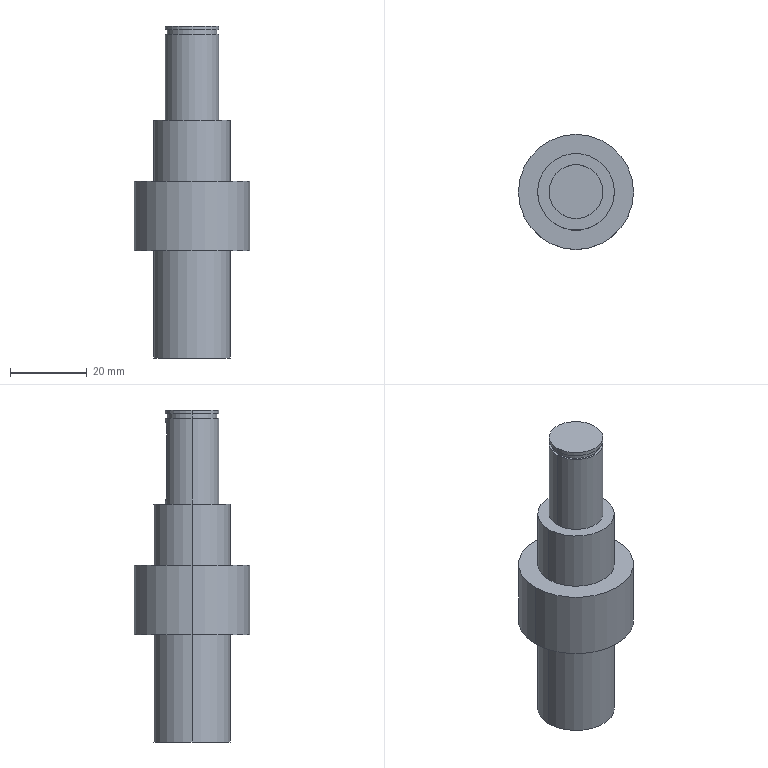Part | STEP file | Push-film main drive shaft SGN-3-03 | 1 solid | 36 faces | box 30 x 30 x 86.5 mm | volume 24651 mm3 | cylinder 21 | plane 15 | commonest cylinder face diameters 14 x7 20 x4 5 x3 17 x3 12.9 x2 30 x2